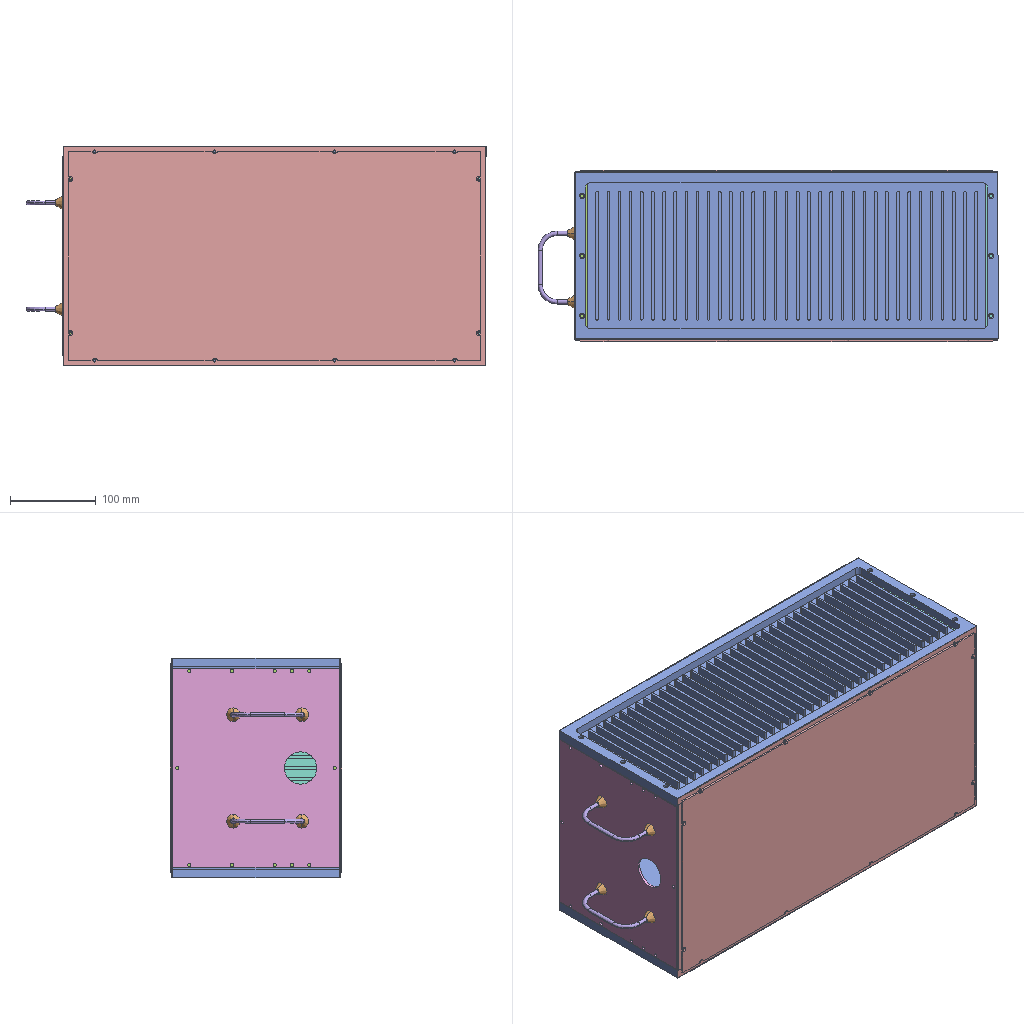Assembly | SolidWorks | 8 different items | 14 placed | box 536 x 200 x 256 mm
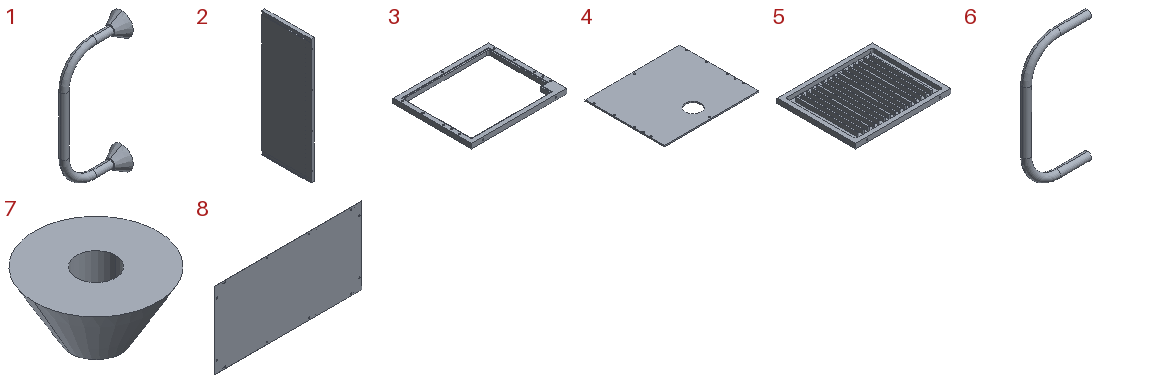Parts list (item | name | quantity | size | volume | features):
1 | (subassembly) | x1 | 42.5 x 15.738 x 95.738 mm | 4133 mm3 | -
2 | - | x2 | 12 x 194 x 493 mm | 496868 mm3 | features ICE 6, MirrorPattern 3, Extrusion 1, Fillet 1, LPattern 1
3 | - | x1 | 236.3 x 194 x 12 mm | 125428 mm3 | features ICE 6, MirrorPattern 3, Extrusion 1, Fillet 1
4 | - | x1 | 232.3 x 194 x 3 mm | 131344 mm3 | features ICE 3, Extrusion 1, MirrorPattern 1
5 | - | x1 | 236.3 x 194 x 12 mm | 243005 mm3 | features ICE 4, MirrorPattern 2, Extrusion 1, Fillet 1, LPattern 1
6 | - | x2 | 42.5 x 5 x 85 mm | 2804 mm3 | features Sweep 1
7 | - | x4 | 15.738 x 15.738 x 8 mm | 664.377 mm3 | features Extrusion 1, ICE 1
8 | - | x2 | 493 x 3 x 256.3 mm | 360860 mm3 | features ICE 4, MirrorPattern 2, Extrusion 1
Mates (type | each side: item.copy, entity, surface, feature):
Coincident | 8.1 plane | assembly plane | 3 times
Coincident | 8.1 face plane Boss-Extrude1 | 2.1 face plane Boss-Extrude1
Concentric | 8.1 face cylinder Mirror1 | 2.1 face cylinder Cut-Extrude4 | 2 times
Coincident | 8.1 face plane Boss-Extrude1 | 3.1 face plane Boss-Extrude1
Coincident | 2.1 face plane Cut-Extrude3 | 3.1 face plane Boss-Extrude1 | 2 times
Coincident | 8.1 face plane Boss-Extrude1 | 2.2 face plane Boss-Extrude1
Concentric | 8.1 face cylinder Cut-Extrude2 | 2.2 face cylinder Cut-Extrude4 | 2 times
Coincident | 2.2 face plane Boss-Extrude1 | 8.2 face plane Boss-Extrude1
Concentric | 2.2 face cylinder Mirror3 | 8.2 face cylinder Cut-Extrude2 | 2 times
Coincident | 3.1 face plane Boss-Extrude1 | 4.1 face plane Boss-Extrude1
Concentric | 3.1 face cylinder Cut-Extrude6 | 4.1 face cylinder Mirror1
Concentric | 3.1 face cylinder Mirror3 | 4.1 face cylinder Cut-Extrude3
Coincident | 2.1 face plane Mirror2 | 5.1 face plane Boss-Extrude1 | 2 times
Coincident | 8.1 face plane Boss-Extrude1 | 5.1 face plane Boss-Extrude1
Coincident | 4.1 face plane Boss-Extrude1 | 7.1 face plane Boss-Extrude1
Parallel | 7.1 plane | assembly plane
Concentric | 7.1 face cylinder Cut-Extrude1 | 6.1 face cylinder Sweep1
Parallel | 6.1 plane | assembly plane
Coincident | 4.1 face plane Boss-Extrude1 | 7.2 face plane Boss-Extrude1
Concentric | 6.1 face cylinder Sweep1 | 7.2 face cylinder Cut-Extrude1
Coincident | 4.1 face plane Boss-Extrude1 | 6.1 face plane Sweep1